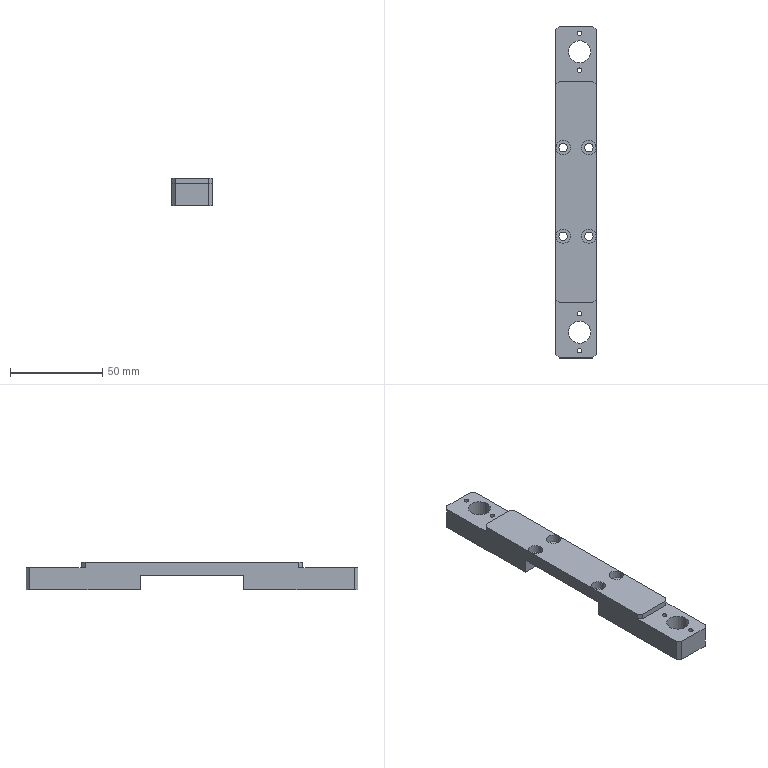Part | NX | 1 solid | 40 faces | box 22 x 180 x 15 mm | volume 41490 mm3 | plane 26 | cylinder 14 | commonest cylinder face diameters 2.5 x4 4.5 x4 7.8 x4 12 x2
STEP:
#1=CARTESIAN_POINT('',(-9.,90.,4.5));
#2=VERTEX_POINT('',#1);
#3=CARTESIAN_POINT('',(-11.,88.,4.5));
#4=VERTEX_POINT('',#3);
#5=CARTESIAN_POINT('',(-11.,88.,4.5));
#6=DIRECTION('',(-0.7071,-0.7071,0.));
#7=VECTOR('',#6,1000.);
#8=LINE('',#5,#7);
#9=EDGE_CURVE('',#2,#4,#8,.T.);
#10=ORIENTED_EDGE('',*,*,#9,.F.);
#11=CARTESIAN_POINT('',(-9.,90.,-7.5));
#12=VERTEX_POINT('',#11);
#13=CARTESIAN_POINT('',(-9.,90.,7.5));
#14=DIRECTION('',(0.,0.,1.));
#15=VECTOR('',#14,1000.);
#16=LINE('',#13,#15);
#17=EDGE_CURVE('',#12,#2,#16,.T.);
#18=ORIENTED_EDGE('',*,*,#17,.F.);
#19=CARTESIAN_POINT('',(-11.,88.,-7.5));
#20=VERTEX_POINT('',#19);
#21=CARTESIAN_POINT('',(-11.,88.,-7.5));
#22=DIRECTION('',(0.7071,0.7071,0.));
#23=VECTOR('',#22,1000.);
#24=LINE('',#21,#23);
#25=EDGE_CURVE('',#20,#12,#24,.T.);
#26=ORIENTED_EDGE('',*,*,#25,.F.);
#27=CARTESIAN_POINT('',(-11.,88.,7.5));
#28=DIRECTION('',(0.,0.,-1.));
#29=VECTOR('',#28,1000.);
#30=LINE('',#27,#29);
#31=EDGE_CURVE('',#4,#20,#30,.T.);
#32=ORIENTED_EDGE('',*,*,#31,.F.);
#33=EDGE_LOOP('',(#10,#18,#26,#32));
#34=FACE_BOUND('',#33,.T.);
#35=CARTESIAN_POINT('',(-11.,88.,7.5));
#36=DIRECTION('',(0.7071,-0.7071,0.));
#37=DIRECTION('',(0.,0.,-1.));
#38=AXIS2_PLACEMENT_3D('',#35,#36,#37);
#39=PLANE('',#38);
#40=ADVANCED_FACE('',(#34),#39,.F.);
#41=CARTESIAN_POINT('',(11.,88.,4.5));
#42=VERTEX_POINT('',#41);
#43=CARTESIAN_POINT('',(9.,90.,4.5));
#44=VERTEX_POINT('',#43);
#45=CARTESIAN_POINT('',(9.,90.,4.5));
#46=DIRECTION('',(-0.7071,0.7071,0.));
#47=VECTOR('',#46,1000.);
#48=LINE('',#45,#47);
#49=EDGE_CURVE('',#42,#44,#48,.T.);
#50=ORIENTED_EDGE('',*,*,#49,.F.);
#51=CARTESIAN_POINT('',(11.,88.,-7.5));
#52=VERTEX_POINT('',#51);
#53=CARTESIAN_POINT('',(11.,88.,7.5));
#54=DIRECTION('',(0.,0.,1.));
#55=VECTOR('',#54,1000.);
#56=LINE('',#53,#55);
#57=EDGE_CURVE('',#52,#42,#56,.T.);
#58=ORIENTED_EDGE('',*,*,#57,.F.);
#59=CARTESIAN_POINT('',(9.,90.,-7.5));
#60=VERTEX_POINT('',#59);
#61=CARTESIAN_POINT('',(9.,90.,-7.5));
#62=DIRECTION('',(0.7071,-0.7071,0.));
#63=VECTOR('',#62,1000.);
#64=LINE('',#61,#63);
#65=EDGE_CURVE('',#60,#52,#64,.T.);
#66=ORIENTED_EDGE('',*,*,#65,.F.);
#67=CARTESIAN_POINT('',(9.,90.,7.5));
#68=DIRECTION('',(0.,0.,-1.));
#69=VECTOR('',#68,1000.);
#70=LINE('',#67,#69);
#71=EDGE_CURVE('',#44,#60,#70,.T.);
#72=ORIENTED_EDGE('',*,*,#71,.F.);
#73=EDGE_LOOP('',(#50,#58,#66,#72));
#74=FACE_BOUND('',#73,.T.);
#75=CARTESIAN_POINT('',(9.,90.,7.5));
#76=DIRECTION('',(-0.7071,-0.7071,0.));
#77=DIRECTION('',(0.,0.,-1.));
#78=AXIS2_PLACEMENT_3D('',#75,#76,#77);
#79=PLANE('',#78);
#80=ADVANCED_FACE('',(#74),#79,.F.);
#81=CARTESIAN_POINT('',(-11.,-88.,4.5));
#82=VERTEX_POINT('',#81);
#83=CARTESIAN_POINT('',(-9.,-90.,4.5));
#84=VERTEX_POINT('',#83);
#85=CARTESIAN_POINT('',(-9.,-90.,4.5));
#86=DIRECTION('',(0.7071,-0.7071,0.));
#87=VECTOR('',#86,1000.);
#88=LINE('',#85,#87);
#89=EDGE_CURVE('',#82,#84,#88,.T.);
#90=ORIENTED_EDGE('',*,*,#89,.F.);
#91=CARTESIAN_POINT('',(-11.,-88.,-7.5));
#92=VERTEX_POINT('',#91);
#93=CARTESIAN_POINT('',(-11.,-88.,7.5));
#94=DIRECTION('',(0.,0.,1.));
#95=VECTOR('',#94,1000.);
#96=LINE('',#93,#95);
#97=EDGE_CURVE('',#92,#82,#96,.T.);
#98=ORIENTED_EDGE('',*,*,#97,.F.);
#99=CARTESIAN_POINT('',(-9.,-90.,-7.5));
#100=VERTEX_POINT('',#99);
#101=CARTESIAN_POINT('',(-9.,-90.,-7.5));
#102=DIRECTION('',(-0.7071,0.7071,0.));
#103=VECTOR('',#102,1000.);
#104=LINE('',#101,#103);
#105=EDGE_CURVE('',#100,#92,#104,.T.);
#106=ORIENTED_EDGE('',*,*,#105,.F.);
#107=CARTESIAN_POINT('',(-9.,-90.,7.5));
#108=DIRECTION('',(0.,0.,-1.));
#109=VECTOR('',#108,1000.);
#110=LINE('',#107,#109);
#111=EDGE_CURVE('',#84,#100,#110,.T.);
#112=ORIENTED_EDGE('',*,*,#111,.F.);
#113=EDGE_LOOP('',(#90,#98,#106,#112));
#114=FACE_BOUND('',#113,.T.);
#115=CARTESIAN_POINT('',(-9.,-90.,7.5));
#116=DIRECTION('',(0.7071,0.7071,0.));
#117=DIRECTION('',(0.,0.,-1.));
#118=AXIS2_PLACEMENT_3D('',#115,#116,#117);
#119=PLANE('',#118);
#120=ADVANCED_FACE('',(#114),#119,.F.);
#121=CARTESIAN_POINT('',(9.,-90.,4.5));
#122=VERTEX_POINT('',#121);
#123=CARTESIAN_POINT('',(11.,-88.,4.5));
#124=VERTEX_POINT('',#123);
#125=CARTESIAN_POINT('',(11.,-88.,4.5));
#126=DIRECTION('',(0.7071,0.7071,0.));
#127=VECTOR('',#126,1000.);
#128=LINE('',#125,#127);
#129=EDGE_CURVE('',#122,#124,#128,.T.);
#130=ORIENTED_EDGE('',*,*,#129,.F.);
#131=CARTESIAN_POINT('',(9.,-90.,-7.5));
#132=VERTEX_POINT('',#131);
#133=CARTESIAN_POINT('',(9.,-90.,7.5));
#134=DIRECTION('',(0.,0.,1.));
#135=VECTOR('',#134,1000.);
#136=LINE('',#133,#135);
#137=EDGE_CURVE('',#132,#122,#136,.T.);
#138=ORIENTED_EDGE('',*,*,#137,.F.);
#139=CARTESIAN_POINT('',(11.,-88.,-7.5));
#140=VERTEX_POINT('',#139);
#141=CARTESIAN_POINT('',(11.,-88.,-7.5));
#142=DIRECTION('',(-0.7071,-0.7071,0.));
#143=VECTOR('',#142,1000.);
#144=LINE('',#141,#143);
#145=EDGE_CURVE('',#140,#132,#144,.T.);
#146=ORIENTED_EDGE('',*,*,#145,.F.);
#147=CARTESIAN_POINT('',(11.,-88.,7.5));
#148=DIRECTION('',(0.,0.,-1.));
#149=VECTOR('',#148,1000.);
#150=LINE('',#147,#149);
#151=EDGE_CURVE('',#124,#140,#150,.T.);
#152=ORIENTED_EDGE('',*,*,#151,.F.);
#153=EDGE_LOOP('',(#130,#138,#146,#152));
#154=FACE_BOUND('',#153,.T.);
#155=CARTESIAN_POINT('',(11.,-88.,7.5));
#156=DIRECTION('',(-0.7071,0.7071,0.));
#157=DIRECTION('',(0.,0.,-1.));
#158=AXIS2_PLACEMENT_3D('',#155,#156,#157);
#159=PLANE('',#158);
#160=ADVANCED_FACE('',(#154),#159,.F.);
#161=CARTESIAN_POINT('',(-9.,-60.,4.5));
#162=VERTEX_POINT('',#161);
#163=CARTESIAN_POINT('',(-11.,-58.,4.5));
#164=VERTEX_POINT('',#163);
#165=CARTESIAN_POINT('',(-34.5,-34.5,4.5));
#166=DIRECTION('',(-0.7071,0.7071,0.));
#167=VECTOR('',#166,1000.);
#168=LINE('',#165,#167);
#169=EDGE_CURVE('',#162,#164,#168,.T.);
#170=ORIENTED_EDGE('',*,*,#169,.F.);
#171=CARTESIAN_POINT('',(-9.,-60.,7.5));
#172=VERTEX_POINT('',#171);
#173=CARTESIAN_POINT('',(-9.,-60.,4.5));
#174=DIRECTION('',(0.,0.,-1.));
#175=VECTOR('',#174,1000.);
#176=LINE('',#173,#175);
#177=EDGE_CURVE('',#172,#162,#176,.T.);
#178=ORIENTED_EDGE('',*,*,#177,.F.);
#179=CARTESIAN_POINT('',(-11.,-58.,7.5));
#180=VERTEX_POINT('',#179);
#181=CARTESIAN_POINT('',(-34.5,-34.5,7.5));
#182=DIRECTION('',(0.7071,-0.7071,0.));
#183=VECTOR('',#182,1000.);
#184=LINE('',#181,#183);
#185=EDGE_CURVE('',#180,#172,#184,.T.);
#186=ORIENTED_EDGE('',*,*,#185,.F.);
#187=CARTESIAN_POINT('',(-11.,-58.,7.5));
#188=DIRECTION('',(0.,0.,1.));
#189=VECTOR('',#188,1000.);
#190=LINE('',#187,#189);
#191=EDGE_CURVE('',#164,#180,#190,.T.);
#192=ORIENTED_EDGE('',*,*,#191,.F.);
#193=EDGE_LOOP('',(#170,#178,#186,#192));
#194=FACE_BOUND('',#193,.T.);
#195=CARTESIAN_POINT('',(-11.,-58.,7.5));
#196=DIRECTION('',(0.7071,0.7071,0.));
#197=DIRECTION('',(0.,0.,1.));
#198=AXIS2_PLACEMENT_3D('',#195,#196,#197);
#199=PLANE('',#198);
#200=ADVANCED_FACE('',(#194),#199,.F.);
#201=CARTESIAN_POINT('',(11.,-58.,4.5));
#202=VERTEX_POINT('',#201);
#203=CARTESIAN_POINT('',(9.,-60.,4.5));
#204=VERTEX_POINT('',#203);
#205=CARTESIAN_POINT('',(34.5,-34.5,4.5));
#206=DIRECTION('',(-0.7071,-0.7071,0.));
#207=VECTOR('',#206,1000.);
#208=LINE('',#205,#207);
#209=EDGE_CURVE('',#202,#204,#208,.T.);
#210=ORIENTED_EDGE('',*,*,#209,.F.);
#211=CARTESIAN_POINT('',(11.,-58.,7.5));
#212=VERTEX_POINT('',#211);
#213=CARTESIAN_POINT('',(11.,-58.,7.5));
#214=DIRECTION('',(0.,0.,-1.));
#215=VECTOR('',#214,1000.);
#216=LINE('',#213,#215);
#217=EDGE_CURVE('',#212,#202,#216,.T.);
#218=ORIENTED_EDGE('',*,*,#217,.F.);
#219=CARTESIAN_POINT('',(9.,-60.,7.5));
#220=VERTEX_POINT('',#219);
#221=CARTESIAN_POINT('',(34.5,-34.5,7.5));
#222=DIRECTION('',(0.7071,0.7071,0.));
#223=VECTOR('',#222,1000.);
#224=LINE('',#221,#223);
#225=EDGE_CURVE('',#220,#212,#224,.T.);
#226=ORIENTED_EDGE('',*,*,#225,.F.);
#227=CARTESIAN_POINT('',(9.,-60.,4.5));
#228=DIRECTION('',(0.,0.,1.));
#229=VECTOR('',#228,1000.);
#230=LINE('',#227,#229);
#231=EDGE_CURVE('',#204,#220,#230,.T.);
#232=ORIENTED_EDGE('',*,*,#231,.F.);
#233=EDGE_LOOP('',(#210,#218,#226,#232));
#234=FACE_BOUND('',#233,.T.);
#235=CARTESIAN_POINT('',(9.,-60.,4.5));
#236=DIRECTION('',(-0.7071,0.7071,0.));
#237=DIRECTION('',(0.,0.,1.));
#238=AXIS2_PLACEMENT_3D('',#235,#236,#237);
#239=PLANE('',#238);
#240=ADVANCED_FACE('',(#234),#239,.F.);
#241=CARTESIAN_POINT('',(-11.,58.,4.5));
#242=VERTEX_POINT('',#241);
#243=CARTESIAN_POINT('',(-9.,60.,4.5));
#244=VERTEX_POINT('',#243);
#245=CARTESIAN_POINT('',(-34.5,34.5,4.5));
#246=DIRECTION('',(0.7071,0.7071,0.));
#247=VECTOR('',#246,1000.);
#248=LINE('',#245,#247);
#249=EDGE_CURVE('',#242,#244,#248,.T.);
#250=ORIENTED_EDGE('',*,*,#249,.F.);
#251=CARTESIAN_POINT('',(-11.,58.,7.5));
#252=VERTEX_POINT('',#251);
#253=CARTESIAN_POINT('',(-11.,58.,7.5));
#254=DIRECTION('',(0.,0.,-1.));
#255=VECTOR('',#254,1000.);
#256=LINE('',#253,#255);
#257=EDGE_CURVE('',#252,#242,#256,.T.);
#258=ORIENTED_EDGE('',*,*,#257,.F.);
#259=CARTESIAN_POINT('',(-9.,60.,7.5));
#260=VERTEX_POINT('',#259);
#261=CARTESIAN_POINT('',(-34.5,34.5,7.5));
#262=DIRECTION('',(-0.7071,-0.7071,0.));
#263=VECTOR('',#262,1000.);
#264=LINE('',#261,#263);
#265=EDGE_CURVE('',#260,#252,#264,.T.);
#266=ORIENTED_EDGE('',*,*,#265,.F.);
#267=CARTESIAN_POINT('',(-9.,60.,4.5));
#268=DIRECTION('',(0.,0.,1.));
#269=VECTOR('',#268,1000.);
#270=LINE('',#267,#269);
#271=EDGE_CURVE('',#244,#260,#270,.T.);
#272=ORIENTED_EDGE('',*,*,#271,.F.);
#273=EDGE_LOOP('',(#250,#258,#266,#272));
#274=FACE_BOUND('',#273,.T.);
#275=CARTESIAN_POINT('',(-9.,60.,4.5));
#276=DIRECTION('',(0.7071,-0.7071,0.));
#277=DIRECTION('',(0.,0.,1.));
#278=AXIS2_PLACEMENT_3D('',#275,#276,#277);
#279=PLANE('',#278);
#280=ADVANCED_FACE('',(#274),#279,.F.);
#281=CARTESIAN_POINT('',(9.,60.,4.5));
#282=VERTEX_POINT('',#281);
#283=CARTESIAN_POINT('',(11.,58.,4.5));
#284=VERTEX_POINT('',#283);
#285=CARTESIAN_POINT('',(34.5,34.5,4.5));
#286=DIRECTION('',(0.7071,-0.7071,0.));
#287=VECTOR('',#286,1000.);
#288=LINE('',#285,#287);
#289=EDGE_CURVE('',#282,#284,#288,.T.);
#290=ORIENTED_EDGE('',*,*,#289,.F.);
#291=CARTESIAN_POINT('',(9.,60.,7.5));
#292=VERTEX_POINT('',#291);
#293=CARTESIAN_POINT('',(9.,60.,4.5));
#294=DIRECTION('',(0.,0.,-1.));
#295=VECTOR('',#294,1000.);
#296=LINE('',#293,#295);
#297=EDGE_CURVE('',#292,#282,#296,.T.);
#298=ORIENTED_EDGE('',*,*,#297,.F.);
#299=CARTESIAN_POINT('',(11.,58.,7.5));
#300=VERTEX_POINT('',#299);
#301=CARTESIAN_POINT('',(34.5,34.5,7.5));
#302=DIRECTION('',(-0.7071,0.7071,0.));
#303=VECTOR('',#302,1000.);
#304=LINE('',#301,#303);
#305=EDGE_CURVE('',#300,#292,#304,.T.);
#306=ORIENTED_EDGE('',*,*,#305,.F.);
#307=CARTESIAN_POINT('',(11.,58.,7.5));
#308=DIRECTION('',(0.,0.,1.));
#309=VECTOR('',#308,1000.);
#310=LINE('',#307,#309);
#311=EDGE_CURVE('',#284,#300,#310,.T.);
#312=ORIENTED_EDGE('',*,*,#311,.F.);
#313=EDGE_LOOP('',(#290,#298,#306,#312));
#314=FACE_BOUND('',#313,.T.);
#315=CARTESIAN_POINT('',(11.,58.,7.5));
#316=DIRECTION('',(-0.7071,-0.7071,0.));
#317=DIRECTION('',(0.,0.,1.));
#318=AXIS2_PLACEMENT_3D('',#315,#316,#317);
#319=PLANE('',#318);
#320=ADVANCED_FACE('',(#314),#319,.F.);
#321=CARTESIAN_POINT('',(-11.,28.05,-7.5));
#322=VERTEX_POINT('',#321);
#323=CARTESIAN_POINT('',(11.,28.05,-7.5));
#324=VERTEX_POINT('',#323);
#325=CARTESIAN_POINT('',(11.,28.05,-7.5));
#326=DIRECTION('',(1.,0.,0.));
#327=VECTOR('',#326,1000.);
#328=LINE('',#325,#327);
#329=EDGE_CURVE('',#322,#324,#328,.T.);
#330=ORIENTED_EDGE('',*,*,#329,.T.);
#331=CARTESIAN_POINT('',(11.,28.05,0.5));
#332=VERTEX_POINT('',#331);
#333=CARTESIAN_POINT('',(11.,28.05,0.5));
#334=DIRECTION('',(0.,0.,-1.));
#335=VECTOR('',#334,1000.);
#336=LINE('',#333,#335);
#337=EDGE_CURVE('',#332,#324,#336,.T.);
#338=ORIENTED_EDGE('',*,*,#337,.F.);
#339=CARTESIAN_POINT('',(-11.,28.05,0.5));
#340=VERTEX_POINT('',#339);
#341=CARTESIAN_POINT('',(11.,28.05,0.5));
#342=DIRECTION('',(1.,0.,0.));
#343=VECTOR('',#342,1000.);
#344=LINE('',#341,#343);
#345=EDGE_CURVE('',#340,#332,#344,.T.);
#346=ORIENTED_EDGE('',*,*,#345,.F.);
#347=CARTESIAN_POINT('',(-11.,28.05,0.5));
#348=DIRECTION('',(0.,0.,-1.));
#349=VECTOR('',#348,1000.);
#350=LINE('',#347,#349);
#351=EDGE_CURVE('',#340,#322,#350,.T.);
#352=ORIENTED_EDGE('',*,*,#351,.T.);
#353=EDGE_LOOP('',(#330,#338,#346,#352));
#354=FACE_BOUND('',#353,.T.);
#355=CARTESIAN_POINT('',(11.,28.05,0.5));
#356=DIRECTION('',(0.,1.,0.));
#357=DIRECTION('',(0.,0.,1.));
#358=AXIS2_PLACEMENT_3D('',#355,#356,#357);
#359=PLANE('',#358);
#360=ADVANCED_FACE('',(#354),#359,.F.);
#361=CARTESIAN_POINT('',(11.,-28.05,-7.5));
#362=VERTEX_POINT('',#361);
#363=CARTESIAN_POINT('',(-11.,-28.05,-7.5));
#364=VERTEX_POINT('',#363);
#365=CARTESIAN_POINT('',(11.,-28.05,-7.5));
#366=DIRECTION('',(-1.,0.,0.));
#367=VECTOR('',#366,1000.);
#368=LINE('',#365,#367);
#369=EDGE_CURVE('',#362,#364,#368,.T.);
#370=ORIENTED_EDGE('',*,*,#369,.T.);
#371=CARTESIAN_POINT('',(-11.,-28.05,0.5));
#372=VERTEX_POINT('',#371);
#373=CARTESIAN_POINT('',(-11.,-28.05,0.5));
#374=DIRECTION('',(0.,0.,-1.));
#375=VECTOR('',#374,1000.);
#376=LINE('',#373,#375);
#377=EDGE_CURVE('',#372,#364,#376,.T.);
#378=ORIENTED_EDGE('',*,*,#377,.F.);
#379=CARTESIAN_POINT('',(11.,-28.05,0.5));
#380=VERTEX_POINT('',#379);
#381=CARTESIAN_POINT('',(11.,-28.05,0.5));
#382=DIRECTION('',(-1.,0.,0.));
#383=VECTOR('',#382,1000.);
#384=LINE('',#381,#383);
#385=EDGE_CURVE('',#380,#372,#384,.T.);
#386=ORIENTED_EDGE('',*,*,#385,.F.);
#387=CARTESIAN_POINT('',(11.,-28.05,0.5));
#388=DIRECTION('',(0.,0.,-1.));
#389=VECTOR('',#388,1000.);
#390=LINE('',#387,#389);
#391=EDGE_CURVE('',#380,#362,#390,.T.);
#392=ORIENTED_EDGE('',*,*,#391,.T.);
#393=EDGE_LOOP('',(#370,#378,#386,#392));
#394=FACE_BOUND('',#393,.T.);
#395=CARTESIAN_POINT('',(11.,-28.05,0.5));
#396=DIRECTION('',(0.,-1.,0.));
#397=DIRECTION('',(0.,0.,-1.));
#398=AXIS2_PLACEMENT_3D('',#395,#396,#397);
#399=PLANE('',#398);
#400=ADVANCED_FACE('',(#394),#399,.F.);
#401=CARTESIAN_POINT('',(-4.75,-24.,0.5));
#402=VERTEX_POINT('',#401);
#403=CARTESIAN_POINT('',(-7.,-24.,0.5));
#404=DIRECTION('',(0.,0.,-1.));
#405=DIRECTION('',(1.,0.,0.));
#406=AXIS2_PLACEMENT_3D('',#403,#404,#405);
#407=CIRCLE('',#406,2.25);
#408=EDGE_CURVE('',#402,#402,#407,.T.);
#409=ORIENTED_EDGE('',*,*,#408,.F.);
#410=EDGE_LOOP('',(#409));
#411=FACE_BOUND('',#410,.T.);
#412=CARTESIAN_POINT('',(9.25,24.,0.5));
#413=VERTEX_POINT('',#412);
#414=CARTESIAN_POINT('',(7.,24.,0.5));
#415=DIRECTION('',(0.,0.,-1.));
#416=DIRECTION('',(1.,0.,0.));
#417=AXIS2_PLACEMENT_3D('',#414,#415,#416);
#418=CIRCLE('',#417,2.25);
#419=EDGE_CURVE('',#413,#413,#418,.T.);
#420=ORIENTED_EDGE('',*,*,#419,.F.);
#421=EDGE_LOOP('',(#420));
#422=FACE_BOUND('',#421,.T.);
#423=CARTESIAN_POINT('',(-11.,-28.05,0.5));
#424=DIRECTION('',(0.,1.,0.));
#425=VECTOR('',#424,1000.);
#426=LINE('',#423,#425);
#427=EDGE_CURVE('',#372,#340,#426,.T.);
#428=ORIENTED_EDGE('',*,*,#427,.T.);
#429=ORIENTED_EDGE('',*,*,#345,.T.);
#430=CARTESIAN_POINT('',(11.,-28.05,0.5));
#431=DIRECTION('',(0.,-1.,0.));
#432=VECTOR('',#431,1000.);
#433=LINE('',#430,#432);
#434=EDGE_CURVE('',#332,#380,#433,.T.);
#435=ORIENTED_EDGE('',*,*,#434,.T.);
#436=ORIENTED_EDGE('',*,*,#385,.T.);
#437=EDGE_LOOP('',(#428,#429,#435,#436));
#438=FACE_BOUND('',#437,.T.);
#439=CARTESIAN_POINT('',(-4.75,24.,0.5));
#440=VERTEX_POINT('',#439);
#441=CARTESIAN_POINT('',(-7.,24.,0.5));
#442=DIRECTION('',(0.,0.,-1.));
#443=DIRECTION('',(1.,0.,0.));
#444=AXIS2_PLACEMENT_3D('',#441,#442,#443);
#445=CIRCLE('',#444,2.25);
#446=EDGE_CURVE('',#440,#440,#445,.T.);
#447=ORIENTED_EDGE('',*,*,#446,.F.);
#448=EDGE_LOOP('',(#447));
#449=FACE_BOUND('',#448,.T.);
#450=CARTESIAN_POINT('',(9.25,-24.,0.5));
#451=VERTEX_POINT('',#450);
#452=CARTESIAN_POINT('',(7.,-24.,0.5));
#453=DIRECTION('',(0.,0.,-1.));
#454=DIRECTION('',(1.,0.,0.));
#455=AXIS2_PLACEMENT_3D('',#452,#453,#454);
#456=CIRCLE('',#455,2.25);
#457=EDGE_CURVE('',#451,#451,#456,.T.);
#458=ORIENTED_EDGE('',*,*,#457,.F.);
#459=EDGE_LOOP('',(#458));
#460=FACE_BOUND('',#459,.T.);
#461=CARTESIAN_POINT('',(0.,0.,0.5));
#462=DIRECTION('',(0.,0.,1.));
#463=DIRECTION('',(1.,0.,0.));
#464=AXIS2_PLACEMENT_3D('',#461,#462,#463);
#465=PLANE('',#464);
#466=ADVANCED_FACE('',(#411,#422,#438,#449,#460),#465,.F.);
#467=CARTESIAN_POINT('',(-11.,60.,7.5));
#468=DIRECTION('',(1.,0.,0.));
#469=VECTOR('',#468,1000.);
#470=LINE('',#467,#469);
#471=EDGE_CURVE('',#260,#292,#470,.T.);
#472=ORIENTED_EDGE('',*,*,#471,.T.);
#473=ORIENTED_EDGE('',*,*,#297,.T.);
#474=CARTESIAN_POINT('',(-11.,60.,4.5));
#475=DIRECTION('',(1.,0.,0.));
#476=VECTOR('',#475,1000.);
#477=LINE('',#474,#476);
#478=EDGE_CURVE('',#244,#282,#477,.T.);
#479=ORIENTED_EDGE('',*,*,#478,.F.);
#480=ORIENTED_EDGE('',*,*,#271,.T.);
#481=EDGE_LOOP('',(#472,#473,#479,#480));
#482=FACE_BOUND('',#481,.T.);
#483=CARTESIAN_POINT('',(-11.,60.,4.5));
#484=DIRECTION('',(0.,-1.,0.));
#485=DIRECTION('',(0.,0.,-1.));
#486=AXIS2_PLACEMENT_3D('',#483,#484,#485);
#487=PLANE('',#486);
#488=ADVANCED_FACE('',(#482),#487,.F.);
#489=CARTESIAN_POINT('',(-4.,76.,4.5));
#490=VERTEX_POINT('',#489);
#491=CARTESIAN_POINT('',(2.,76.,4.5));
#492=DIRECTION('',(0.,0.,1.));
#493=DIRECTION('',(-1.,0.,0.));
#494=AXIS2_PLACEMENT_3D('',#491,#492,#493);
#495=CIRCLE('',#494,6.);
#496=EDGE_CURVE('',#490,#490,#495,.T.);
#497=ORIENTED_EDGE('',*,*,#496,.F.);
#498=EDGE_LOOP('',(#497));
#499=FACE_BOUND('',#498,.T.);
#500=CARTESIAN_POINT('',(11.,90.,4.5));
#501=DIRECTION('',(0.,1.,0.));
#502=VECTOR('',#501,1000.);
#503=LINE('',#500,#502);
#504=EDGE_CURVE('',#284,#42,#503,.T.);
#505=ORIENTED_EDGE('',*,*,#504,.T.);
#506=ORIENTED_EDGE('',*,*,#49,.T.);
#507=CARTESIAN_POINT('',(-11.,90.,4.5));
#508=DIRECTION('',(-1.,0.,0.));
#509=VECTOR('',#508,1000.);
#510=LINE('',#507,#509);
#511=EDGE_CURVE('',#44,#2,#510,.T.);
#512=ORIENTED_EDGE('',*,*,#511,.T.);
#513=ORIENTED_EDGE('',*,*,#9,.T.);
#514=CARTESIAN_POINT('',(-11.,90.,4.5));
#515=DIRECTION('',(0.,-1.,0.));
#516=VECTOR('',#515,1000.);
#517=LINE('',#514,#516);
#518=EDGE_CURVE('',#4,#242,#517,.T.);
#519=ORIENTED_EDGE('',*,*,#518,.T.);
#520=ORIENTED_EDGE('',*,*,#249,.T.);
#521=ORIENTED_EDGE('',*,*,#478,.T.);
#522=ORIENTED_EDGE('',*,*,#289,.T.);
#523=EDGE_LOOP('',(#505,#506,#512,#513,#519,#520,#521,#522));
#524=FACE_BOUND('',#523,.T.);
#525=CARTESIAN_POINT('',(0.75,66.,4.5));
#526=VERTEX_POINT('',#525);
#527=CARTESIAN_POINT('',(2.,66.,4.5));
#528=DIRECTION('',(0.,0.,-1.));
#529=DIRECTION('',(-1.,0.,0.));
#530=AXIS2_PLACEMENT_3D('',#527,#528,#529);
#531=CIRCLE('',#530,1.25);
#532=EDGE_CURVE('',#526,#526,#531,.T.);
#533=ORIENTED_EDGE('',*,*,#532,.T.);
#534=EDGE_LOOP('',(#533));
#535=FACE_BOUND('',#534,.T.);
#536=CARTESIAN_POINT('',(0.75,86.,4.5));
#537=VERTEX_POINT('',#536);
#538=CARTESIAN_POINT('',(2.,86.,4.5));
#539=DIRECTION('',(0.,0.,-1.));
#540=DIRECTION('',(-1.,0.,0.));
#541=AXIS2_PLACEMENT_3D('',#538,#539,#540);
#542=CIRCLE('',#541,1.25);
#543=EDGE_CURVE('',#537,#537,#542,.T.);
#544=ORIENTED_EDGE('',*,*,#543,.T.);
#545=EDGE_LOOP('',(#544));
#546=FACE_BOUND('',#545,.T.);
#547=CARTESIAN_POINT('',(0.,0.,4.5));
#548=DIRECTION('',(0.,0.,-1.));
#549=DIRECTION('',(-1.,0.,0.));
#550=AXIS2_PLACEMENT_3D('',#547,#548,#549);
#551=PLANE('',#550);
#552=ADVANCED_FACE('',(#499,#524,#535,#546),#551,.F.);
#553=CARTESIAN_POINT('',(-11.,-60.,4.5));
#554=DIRECTION('',(-1.,0.,0.));
#555=VECTOR('',#554,1000.);
#556=LINE('',#553,#555);
#557=EDGE_CURVE('',#204,#162,#556,.T.);
#558=ORIENTED_EDGE('',*,*,#557,.F.);
#559=ORIENTED_EDGE('',*,*,#231,.T.);
#560=CARTESIAN_POINT('',(-11.,-60.,7.5));
#561=DIRECTION('',(-1.,0.,0.));
#562=VECTOR('',#561,1000.);
#563=LINE('',#560,#562);
#564=EDGE_CURVE('',#220,#172,#563,.T.);
#565=ORIENTED_EDGE('',*,*,#564,.T.);
#566=ORIENTED_EDGE('',*,*,#177,.T.);
#567=EDGE_LOOP('',(#558,#559,#565,#566));
#568=FACE_BOUND('',#567,.T.);
#569=CARTESIAN_POINT('',(-11.,-60.,4.5));
#570=DIRECTION('',(0.,1.,0.));
#571=DIRECTION('',(0.,0.,1.));
#572=AXIS2_PLACEMENT_3D('',#569,#570,#571);
#573=PLANE('',#572);
#574=ADVANCED_FACE('',(#568),#573,.F.);
#575=CARTESIAN_POINT('',(-4.,-76.,4.5));
#576=VERTEX_POINT('',#575);
#577=CARTESIAN_POINT('',(2.,-76.,4.5));
#578=DIRECTION('',(0.,0.,1.));
#579=DIRECTION('',(-1.,0.,0.));
#580=AXIS2_PLACEMENT_3D('',#577,#578,#579);
#581=CIRCLE('',#580,6.);
#582=EDGE_CURVE('',#576,#576,#581,.T.);
#583=ORIENTED_EDGE('',*,*,#582,.F.);
#584=EDGE_LOOP('',(#583));
#585=FACE_BOUND('',#584,.T.);
#586=CARTESIAN_POINT('',(-11.,-90.,4.5));
#587=DIRECTION('',(1.,0.,0.));
#588=VECTOR('',#587,1000.);
#589=LINE('',#586,#588);
#590=EDGE_CURVE('',#84,#122,#589,.T.);
#591=ORIENTED_EDGE('',*,*,#590,.T.);
#592=ORIENTED_EDGE('',*,*,#129,.T.);
#593=CARTESIAN_POINT('',(11.,-90.,4.5));
#594=DIRECTION('',(0.,1.,0.));
#595=VECTOR('',#594,1000.);
#596=LINE('',#593,#595);
#597=EDGE_CURVE('',#124,#202,#596,.T.);
#598=ORIENTED_EDGE('',*,*,#597,.T.);
#599=ORIENTED_EDGE('',*,*,#209,.T.);
#600=ORIENTED_EDGE('',*,*,#557,.T.);
#601=ORIENTED_EDGE('',*,*,#169,.T.);
#602=CARTESIAN_POINT('',(-11.,-90.,4.5));
#603=DIRECTION('',(0.,-1.,0.));
#604=VECTOR('',#603,1000.);
#605=LINE('',#602,#604);
#606=EDGE_CURVE('',#164,#82,#605,.T.);
#607=ORIENTED_EDGE('',*,*,#606,.T.);
#608=ORIENTED_EDGE('',*,*,#89,.T.);
#609=EDGE_LOOP('',(#591,#592,#598,#599,#600,#601,#607,#608));
#610=FACE_BOUND('',#609,.T.);
#611=CARTESIAN_POINT('',(0.75,-86.,4.5));
#612=VERTEX_POINT('',#611);
#613=CARTESIAN_POINT('',(2.,-86.,4.5));
#614=DIRECTION('',(0.,0.,-1.));
#615=DIRECTION('',(-1.,0.,0.));
#616=AXIS2_PLACEMENT_3D('',#613,#614,#615);
#617=CIRCLE('',#616,1.25);
#618=EDGE_CURVE('',#612,#612,#617,.T.);
#619=ORIENTED_EDGE('',*,*,#618,.T.);
#620=EDGE_LOOP('',(#619));
#621=FACE_BOUND('',#620,.T.);
#622=CARTESIAN_POINT('',(0.75,-66.,4.5));
#623=VERTEX_POINT('',#622);
#624=CARTESIAN_POINT('',(2.,-66.,4.5));
#625=DIRECTION('',(0.,0.,-1.));
#626=DIRECTION('',(-1.,0.,0.));
#627=AXIS2_PLACEMENT_3D('',#624,#625,#626);
#628=CIRCLE('',#627,1.25);
#629=EDGE_CURVE('',#623,#623,#628,.T.);
#630=ORIENTED_EDGE('',*,*,#629,.T.);
#631=EDGE_LOOP('',(#630));
#632=FACE_BOUND('',#631,.T.);
#633=CARTESIAN_POINT('',(0.,0.,4.5));
#634=DIRECTION('',(0.,0.,-1.));
#635=DIRECTION('',(-1.,0.,0.));
#636=AXIS2_PLACEMENT_3D('',#633,#634,#635);
#637=PLANE('',#636);
#638=ADVANCED_FACE('',(#585,#610,#621,#632),#637,.F.);
#639=CARTESIAN_POINT('',(-10.9,24.,3.1));
#640=VERTEX_POINT('',#639);
#641=CARTESIAN_POINT('',(-7.,24.,3.1));
#642=DIRECTION('',(0.,0.,1.));
#643=DIRECTION('',(-1.,0.,0.));
#644=AXIS2_PLACEMENT_3D('',#641,#642,#643);
#645=CIRCLE('',#644,3.9);
#646=EDGE_CURVE('',#640,#640,#645,.T.);
#647=ORIENTED_EDGE('',*,*,#646,.T.);
#648=EDGE_LOOP('',(#647));
#649=FACE_BOUND('',#648,.T.);
#650=CARTESIAN_POINT('',(-9.25,24.,3.1));
#651=VERTEX_POINT('',#650);
#652=CARTESIAN_POINT('',(-7.,24.,3.1));
#653=DIRECTION('',(0.,0.,1.));
#654=DIRECTION('',(-1.,0.,0.));
#655=AXIS2_PLACEMENT_3D('',#652,#653,#654);
#656=CIRCLE('',#655,2.25);
#657=EDGE_CURVE('',#651,#651,#656,.T.);
#658=ORIENTED_EDGE('',*,*,#657,.F.);
#659=EDGE_LOOP('',(#658));
#660=FACE_BOUND('',#659,.T.);
#661=CARTESIAN_POINT('',(-4.75,-24.,3.1));
#662=DIRECTION('',(0.,0.,-1.));
#663=DIRECTION('',(-1.,0.,0.));
#664=AXIS2_PLACEMENT_3D('',#661,#662,#663);
#665=PLANE('',#664);
#666=ADVANCED_FACE('',(#649,#660),#665,.F.);
#667=CARTESIAN_POINT('',(3.1,24.,3.1));
#668=VERTEX_POINT('',#667);
#669=CARTESIAN_POINT('',(7.,24.,3.1));
#670=DIRECTION('',(0.,0.,1.));
#671=DIRECTION('',(-1.,0.,0.));
#672=AXIS2_PLACEMENT_3D('',#669,#670,#671);
#673=CIRCLE('',#672,3.9);
#674=EDGE_CURVE('',#668,#668,#673,.T.);
#675=ORIENTED_EDGE('',*,*,#674,.T.);
#676=EDGE_LOOP('',(#675));
#677=FACE_BOUND('',#676,.T.);
#678=CARTESIAN_POINT('',(4.75,24.,3.1));
#679=VERTEX_POINT('',#678);
#680=CARTESIAN_POINT('',(7.,24.,3.1));
#681=DIRECTION('',(0.,0.,1.));
#682=DIRECTION('',(-1.,0.,0.));
#683=AXIS2_PLACEMENT_3D('',#680,#681,#682);
#684=CIRCLE('',#683,2.25);
#685=EDGE_CURVE('',#679,#679,#684,.T.);
#686=ORIENTED_EDGE('',*,*,#685,.F.);
#687=EDGE_LOOP('',(#686));
#688=FACE_BOUND('',#687,.T.);
#689=CARTESIAN_POINT('',(-4.75,-24.,3.1));
#690=DIRECTION('',(0.,0.,-1.));
#691=DIRECTION('',(-1.,0.,0.));
#692=AXIS2_PLACEMENT_3D('',#689,#690,#691);
#693=PLANE('',#692);
#694=ADVANCED_FACE('',(#677,#688),#693,.F.);
#695=CARTESIAN_POINT('',(3.1,-24.,3.1));
#696=VERTEX_POINT('',#695);
#697=CARTESIAN_POINT('',(7.,-24.,3.1));
#698=DIRECTION('',(0.,0.,1.));
#699=DIRECTION('',(-1.,0.,0.));
#700=AXIS2_PLACEMENT_3D('',#697,#698,#699);
#701=CIRCLE('',#700,3.9);
#702=EDGE_CURVE('',#696,#696,#701,.T.);
#703=ORIENTED_EDGE('',*,*,#702,.T.);
#704=EDGE_LOOP('',(#703));
#705=FACE_BOUND('',#704,.T.);
#706=CARTESIAN_POINT('',(4.75,-24.,3.1));
#707=VERTEX_POINT('',#706);
#708=CARTESIAN_POINT('',(7.,-24.,3.1));
#709=DIRECTION('',(0.,0.,1.));
#710=DIRECTION('',(-1.,0.,0.));
#711=AXIS2_PLACEMENT_3D('',#708,#709,#710);
#712=CIRCLE('',#711,2.25);
#713=EDGE_CURVE('',#707,#707,#712,.T.);
#714=ORIENTED_EDGE('',*,*,#713,.F.);
#715=EDGE_LOOP('',(#714));
#716=FACE_BOUND('',#715,.T.);
#717=CARTESIAN_POINT('',(-4.75,-24.,3.1));
#718=DIRECTION('',(0.,0.,-1.));
#719=DIRECTION('',(-1.,0.,0.));
#720=AXIS2_PLACEMENT_3D('',#717,#718,#719);
#721=PLANE('',#720);
#722=ADVANCED_FACE('',(#705,#716),#721,.F.);
#723=CARTESIAN_POINT('',(-3.1,-24.,3.1));
#724=VERTEX_POINT('',#723);
#725=CARTESIAN_POINT('',(-7.,-24.,3.1));
#726=DIRECTION('',(0.,0.,1.));
#727=DIRECTION('',(1.,0.,0.));
#728=AXIS2_PLACEMENT_3D('',#725,#726,#727);
#729=CIRCLE('',#728,3.9);
#730=EDGE_CURVE('',#724,#724,#729,.T.);
#731=ORIENTED_EDGE('',*,*,#730,.T.);
#732=EDGE_LOOP('',(#731));
#733=FACE_BOUND('',#732,.T.);
#734=CARTESIAN_POINT('',(-4.75,-24.,3.1));
#735=VERTEX_POINT('',#734);
#736=CARTESIAN_POINT('',(-7.,-24.,3.1));
#737=DIRECTION('',(0.,0.,1.));
#738=DIRECTION('',(1.,0.,0.));
#739=AXIS2_PLACEMENT_3D('',#736,#737,#738);
#740=CIRCLE('',#739,2.25);
#741=EDGE_CURVE('',#735,#735,#740,.T.);
#742=ORIENTED_EDGE('',*,*,#741,.F.);
#743=EDGE_LOOP('',(#742));
#744=FACE_BOUND('',#743,.T.);
#745=CARTESIAN_POINT('',(-4.75,-24.,3.1));
#746=DIRECTION('',(0.,0.,-1.));
#747=DIRECTION('',(-1.,0.,0.));
#748=AXIS2_PLACEMENT_3D('',#745,#746,#747);
#749=PLANE('',#748);
#750=ADVANCED_FACE('',(#733,#744),#749,.F.);
#751=CARTESIAN_POINT('',(-11.,90.,-7.5));
#752=DIRECTION('',(-1.,0.,0.));
#753=VECTOR('',#752,1000.);
#754=LINE('',#751,#753);
#755=EDGE_CURVE('',#60,#12,#754,.T.);
#756=ORIENTED_EDGE('',*,*,#755,.F.);
#757=ORIENTED_EDGE('',*,*,#65,.T.);
#758=CARTESIAN_POINT('',(11.,90.,-7.5));
#759=DIRECTION('',(0.,1.,0.));
#760=VECTOR('',#759,1000.);
#761=LINE('',#758,#760);
#762=EDGE_CURVE('',#324,#52,#761,.T.);
#763=ORIENTED_EDGE('',*,*,#762,.F.);
#764=ORIENTED_EDGE('',*,*,#329,.F.);
#765=CARTESIAN_POINT('',(-11.,90.,-7.5));
#766=DIRECTION('',(0.,-1.,0.));
#767=VECTOR('',#766,1000.);
#768=LINE('',#765,#767);
#769=EDGE_CURVE('',#20,#322,#768,.T.);
#770=ORIENTED_EDGE('',*,*,#769,.F.);
#771=ORIENTED_EDGE('',*,*,#25,.T.);
#772=EDGE_LOOP('',(#756,#757,#763,#764,#770,#771));
#773=FACE_BOUND('',#772,.T.);
#774=CARTESIAN_POINT('',(-4.,76.,-7.5));
#775=VERTEX_POINT('',#774);
#776=CARTESIAN_POINT('',(2.,76.,-7.5));
#777=DIRECTION('',(0.,0.,1.));
#778=DIRECTION('',(-1.,0.,0.));
#779=AXIS2_PLACEMENT_3D('',#776,#777,#778);
#780=CIRCLE('',#779,6.);
#781=EDGE_CURVE('',#775,#775,#780,.T.);
#782=ORIENTED_EDGE('',*,*,#781,.T.);
#783=EDGE_LOOP('',(#782));
#784=FACE_BOUND('',#783,.T.);
#785=CARTESIAN_POINT('',(0.75,66.,-7.5));
#786=VERTEX_POINT('',#785);
#787=CARTESIAN_POINT('',(2.,66.,-7.5));
#788=DIRECTION('',(0.,0.,-1.));
#789=DIRECTION('',(-1.,0.,0.));
#790=AXIS2_PLACEMENT_3D('',#787,#788,#789);
#791=CIRCLE('',#790,1.25);
#792=EDGE_CURVE('',#786,#786,#791,.T.);
#793=ORIENTED_EDGE('',*,*,#792,.F.);
#794=EDGE_LOOP('',(#793));
#795=FACE_BOUND('',#794,.T.);
#796=CARTESIAN_POINT('',(0.75,86.,-7.5));
#797=VERTEX_POINT('',#796);
#798=CARTESIAN_POINT('',(2.,86.,-7.5));
#799=DIRECTION('',(0.,0.,-1.));
#800=DIRECTION('',(-1.,0.,0.));
#801=AXIS2_PLACEMENT_3D('',#798,#799,#800);
#802=CIRCLE('',#801,1.25);
#803=EDGE_CURVE('',#797,#797,#802,.T.);
#804=ORIENTED_EDGE('',*,*,#803,.F.);
#805=EDGE_LOOP('',(#804));
#806=FACE_BOUND('',#805,.T.);
#807=CARTESIAN_POINT('',(0.,0.,-7.5));
#808=DIRECTION('',(0.,0.,1.));
#809=DIRECTION('',(1.,0.,0.));
#810=AXIS2_PLACEMENT_3D('',#807,#808,#809);
#811=PLANE('',#810);
#812=ADVANCED_FACE('',(#773,#784,#795,#806),#811,.F.);
#813=CARTESIAN_POINT('',(-3.1,-24.,7.5));
#814=VERTEX_POINT('',#813);
#815=CARTESIAN_POINT('',(-7.,-24.,7.5));
#816=DIRECTION('',(0.,0.,1.));
#817=DIRECTION('',(1.,0.,0.));
#818=AXIS2_PLACEMENT_3D('',#815,#816,#817);
#819=CIRCLE('',#818,3.9);
#820=EDGE_CURVE('',#814,#814,#819,.T.);
#821=ORIENTED_EDGE('',*,*,#820,.F.);
#822=EDGE_LOOP('',(#821));
#823=FACE_BOUND('',#822,.T.);
#824=CARTESIAN_POINT('',(10.9,-24.,7.5));
#825=VERTEX_POINT('',#824);
#826=CARTESIAN_POINT('',(7.,-24.,7.5));
#827=DIRECTION('',(0.,0.,1.));
#828=DIRECTION('',(1.,0.,0.));
#829=AXIS2_PLACEMENT_3D('',#826,#827,#828);
#830=CIRCLE('',#829,3.9);
#831=EDGE_CURVE('',#825,#825,#830,.T.);
#832=ORIENTED_EDGE('',*,*,#831,.F.);
#833=EDGE_LOOP('',(#832));
#834=FACE_BOUND('',#833,.T.);
#835=CARTESIAN_POINT('',(10.9,24.,7.5));
#836=VERTEX_POINT('',#835);
#837=CARTESIAN_POINT('',(7.,24.,7.5));
#838=DIRECTION('',(0.,0.,1.));
#839=DIRECTION('',(1.,0.,0.));
#840=AXIS2_PLACEMENT_3D('',#837,#838,#839);
#841=CIRCLE('',#840,3.9);
#842=EDGE_CURVE('',#836,#836,#841,.T.);
#843=ORIENTED_EDGE('',*,*,#842,.F.);
#844=EDGE_LOOP('',(#843));
#845=FACE_BOUND('',#844,.T.);
#846=CARTESIAN_POINT('',(-3.1,24.,7.5));
#847=VERTEX_POINT('',#846);
#848=CARTESIAN_POINT('',(-7.,24.,7.5));
#849=DIRECTION('',(0.,0.,1.));
#850=DIRECTION('',(1.,0.,0.));
#851=AXIS2_PLACEMENT_3D('',#848,#849,#850);
#852=CIRCLE('',#851,3.9);
#853=EDGE_CURVE('',#847,#847,#852,.T.);
#854=ORIENTED_EDGE('',*,*,#853,.F.);
#855=EDGE_LOOP('',(#854));
#856=FACE_BOUND('',#855,.T.);
#857=CARTESIAN_POINT('',(11.,90.,7.5));
#858=DIRECTION('',(0.,1.,0.));
#859=VECTOR('',#858,1000.);
#860=LINE('',#857,#859);
#861=EDGE_CURVE('',#212,#300,#860,.T.);
#862=ORIENTED_EDGE('',*,*,#861,.T.);
#863=ORIENTED_EDGE('',*,*,#305,.T.);
#864=ORIENTED_EDGE('',*,*,#471,.F.);
#865=ORIENTED_EDGE('',*,*,#265,.T.);
#866=CARTESIAN_POINT('',(-11.,90.,7.5));
#867=DIRECTION('',(0.,-1.,0.));
#868=VECTOR('',#867,1000.);
#869=LINE('',#866,#868);
#870=EDGE_CURVE('',#252,#180,#869,.T.);
#871=ORIENTED_EDGE('',*,*,#870,.T.);
#872=ORIENTED_EDGE('',*,*,#185,.T.);
#873=ORIENTED_EDGE('',*,*,#564,.F.);
#874=ORIENTED_EDGE('',*,*,#225,.T.);
#875=EDGE_LOOP('',(#862,#863,#864,#865,#871,#872,#873,#874));
#876=FACE_BOUND('',#875,.T.);
#877=CARTESIAN_POINT('',(0.,0.,7.5));
#878=DIRECTION('',(0.,0.,1.));
#879=DIRECTION('',(1.,0.,0.));
#880=AXIS2_PLACEMENT_3D('',#877,#878,#879);
#881=PLANE('',#880);
#882=ADVANCED_FACE('',(#823,#834,#845,#856,#876),#881,.T.);
#883=CARTESIAN_POINT('',(-11.,-90.,-7.5));
#884=DIRECTION('',(1.,0.,0.));
#885=VECTOR('',#884,1000.);
#886=LINE('',#883,#885);
#887=EDGE_CURVE('',#100,#132,#886,.T.);
#888=ORIENTED_EDGE('',*,*,#887,.T.);
#889=ORIENTED_EDGE('',*,*,#137,.T.);
#890=ORIENTED_EDGE('',*,*,#590,.F.);
#891=ORIENTED_EDGE('',*,*,#111,.T.);
#892=EDGE_LOOP('',(#888,#889,#890,#891));
#893=FACE_BOUND('',#892,.T.);
#894=CARTESIAN_POINT('',(-11.,-90.,7.5));
#895=DIRECTION('',(0.,1.,0.));
#896=DIRECTION('',(0.,0.,1.));
#897=AXIS2_PLACEMENT_3D('',#894,#895,#896);
#898=PLANE('',#897);
#899=ADVANCED_FACE('',(#893),#898,.F.);
#900=ORIENTED_EDGE('',*,*,#870,.F.);
#901=ORIENTED_EDGE('',*,*,#257,.T.);
#902=ORIENTED_EDGE('',*,*,#518,.F.);
#903=ORIENTED_EDGE('',*,*,#31,.T.);
#904=ORIENTED_EDGE('',*,*,#769,.T.);
#905=ORIENTED_EDGE('',*,*,#351,.F.);
#906=ORIENTED_EDGE('',*,*,#427,.F.);
#907=ORIENTED_EDGE('',*,*,#377,.T.);
#908=CARTESIAN_POINT('',(-11.,90.,-7.5));
#909=DIRECTION('',(0.,-1.,0.));
#910=VECTOR('',#909,1000.);
#911=LINE('',#908,#910);
#912=EDGE_CURVE('',#364,#92,#911,.T.);
#913=ORIENTED_EDGE('',*,*,#912,.T.);
#914=ORIENTED_EDGE('',*,*,#97,.T.);
#915=ORIENTED_EDGE('',*,*,#606,.F.);
#916=ORIENTED_EDGE('',*,*,#191,.T.);
#917=EDGE_LOOP('',(#900,#901,#902,#903,#904,#905,#906,#907,#913,#914,#915,#916));
#918=FACE_BOUND('',#917,.T.);
#919=CARTESIAN_POINT('',(-11.,90.,7.5));
#920=DIRECTION('',(1.,0.,0.));
#921=DIRECTION('',(0.,1.,0.));
#922=AXIS2_PLACEMENT_3D('',#919,#920,#921);
#923=PLANE('',#922);
#924=ADVANCED_FACE('',(#918),#923,.F.);
#925=ORIENTED_EDGE('',*,*,#511,.F.);
#926=ORIENTED_EDGE('',*,*,#71,.T.);
#927=ORIENTED_EDGE('',*,*,#755,.T.);
#928=ORIENTED_EDGE('',*,*,#17,.T.);
#929=EDGE_LOOP('',(#925,#926,#927,#928));
#930=FACE_BOUND('',#929,.T.);
#931=CARTESIAN_POINT('',(-11.,90.,7.5));
#932=DIRECTION('',(0.,-1.,0.));
#933=DIRECTION('',(0.,0.,-1.));
#934=AXIS2_PLACEMENT_3D('',#931,#932,#933);
#935=PLANE('',#934);
#936=ADVANCED_FACE('',(#930),#935,.F.);
#937=ORIENTED_EDGE('',*,*,#504,.F.);
#938=ORIENTED_EDGE('',*,*,#311,.T.);
#939=ORIENTED_EDGE('',*,*,#861,.F.);
#940=ORIENTED_EDGE('',*,*,#217,.T.);
#941=ORIENTED_EDGE('',*,*,#597,.F.);
#942=ORIENTED_EDGE('',*,*,#151,.T.);
#943=CARTESIAN_POINT('',(11.,90.,-7.5));
#944=DIRECTION('',(0.,1.,0.));
#945=VECTOR('',#944,1000.);
#946=LINE('',#943,#945);
#947=EDGE_CURVE('',#140,#362,#946,.T.);
#948=ORIENTED_EDGE('',*,*,#947,.T.);
#949=ORIENTED_EDGE('',*,*,#391,.F.);
#950=ORIENTED_EDGE('',*,*,#434,.F.);
#951=ORIENTED_EDGE('',*,*,#337,.T.);
#952=ORIENTED_EDGE('',*,*,#762,.T.);
#953=ORIENTED_EDGE('',*,*,#57,.T.);
#954=EDGE_LOOP('',(#937,#938,#939,#940,#941,#942,#948,#949,#950,#951,#952,#953));
#955=FACE_BOUND('',#954,.T.);
#956=CARTESIAN_POINT('',(11.,90.,7.5));
#957=DIRECTION('',(-1.,0.,0.));
#958=DIRECTION('',(0.,-1.,0.));
#959=AXIS2_PLACEMENT_3D('',#956,#957,#958);
#960=PLANE('',#959);
#961=ADVANCED_FACE('',(#955),#960,.F.);
#962=ORIENTED_EDGE('',*,*,#947,.F.);
#963=ORIENTED_EDGE('',*,*,#145,.T.);
#964=ORIENTED_EDGE('',*,*,#887,.F.);
#965=ORIENTED_EDGE('',*,*,#105,.T.);
#966=ORIENTED_EDGE('',*,*,#912,.F.);
#967=ORIENTED_EDGE('',*,*,#369,.F.);
#968=EDGE_LOOP('',(#962,#963,#964,#965,#966,#967));
#969=FACE_BOUND('',#968,.T.);
#970=CARTESIAN_POINT('',(0.75,-66.,-7.5));
#971=VERTEX_POINT('',#970);
#972=CARTESIAN_POINT('',(2.,-66.,-7.5));
#973=DIRECTION('',(0.,0.,-1.));
#974=DIRECTION('',(-1.,0.,0.));
#975=AXIS2_PLACEMENT_3D('',#972,#973,#974);
#976=CIRCLE('',#975,1.25);
#977=EDGE_CURVE('',#971,#971,#976,.T.);
#978=ORIENTED_EDGE('',*,*,#977,.F.);
#979=EDGE_LOOP('',(#978));
#980=FACE_BOUND('',#979,.T.);
#981=CARTESIAN_POINT('',(0.75,-86.,-7.5));
#982=VERTEX_POINT('',#981);
#983=CARTESIAN_POINT('',(2.,-86.,-7.5));
#984=DIRECTION('',(0.,0.,-1.));
#985=DIRECTION('',(-1.,0.,0.));
#986=AXIS2_PLACEMENT_3D('',#983,#984,#985);
#987=CIRCLE('',#986,1.25);
#988=EDGE_CURVE('',#982,#982,#987,.T.);
#989=ORIENTED_EDGE('',*,*,#988,.F.);
#990=EDGE_LOOP('',(#989));
#991=FACE_BOUND('',#990,.T.);
#992=CARTESIAN_POINT('',(8.,-76.,-7.5));
#993=VERTEX_POINT('',#992);
#994=CARTESIAN_POINT('',(2.,-76.,-7.5));
#995=DIRECTION('',(0.,0.,1.));
#996=DIRECTION('',(1.,0.,0.));
#997=AXIS2_PLACEMENT_3D('',#994,#995,#996);
#998=CIRCLE('',#997,6.);
#999=EDGE_CURVE('',#993,#993,#998,.T.);
#1000=ORIENTED_EDGE('',*,*,#999,.T.);
#1001=EDGE_LOOP('',(#1000));
#1002=FACE_BOUND('',#1001,.T.);
#1003=CARTESIAN_POINT('',(0.,0.,-7.5));
#1004=DIRECTION('',(0.,0.,1.));
#1005=DIRECTION('',(1.,0.,0.));
#1006=AXIS2_PLACEMENT_3D('',#1003,#1004,#1005);
#1007=PLANE('',#1006);
#1008=ADVANCED_FACE('',(#969,#980,#991,#1002),#1007,.F.);
#1009=ORIENTED_EDGE('',*,*,#408,.T.);
#1010=EDGE_LOOP('',(#1009));
#1011=FACE_BOUND('',#1010,.T.);
#1012=ORIENTED_EDGE('',*,*,#741,.T.);
#1013=EDGE_LOOP('',(#1012));
#1014=FACE_BOUND('',#1013,.T.);
#1015=CARTESIAN_POINT('',(-7.,-24.,7.5));
#1016=DIRECTION('',(0.,0.,1.));
#1017=DIRECTION('',(1.,0.,0.));
#1018=AXIS2_PLACEMENT_3D('',#1015,#1016,#1017);
#1019=CYLINDRICAL_SURFACE('',#1018,2.25);
#1020=ADVANCED_FACE('',(#1011,#1014),#1019,.F.);
#1021=ORIENTED_EDGE('',*,*,#730,.F.);
#1022=EDGE_LOOP('',(#1021));
#1023=FACE_BOUND('',#1022,.T.);
#1024=ORIENTED_EDGE('',*,*,#820,.T.);
#1025=EDGE_LOOP('',(#1024));
#1026=FACE_BOUND('',#1025,.T.);
#1027=CARTESIAN_POINT('',(-7.,-24.,7.5));
#1028=DIRECTION('',(0.,0.,1.));
#1029=DIRECTION('',(1.,0.,0.));
#1030=AXIS2_PLACEMENT_3D('',#1027,#1028,#1029);
#1031=CYLINDRICAL_SURFACE('',#1030,3.9);
#1032=ADVANCED_FACE('',(#1023,#1026),#1031,.F.);
#1033=ORIENTED_EDGE('',*,*,#457,.T.);
#1034=EDGE_LOOP('',(#1033));
#1035=FACE_BOUND('',#1034,.T.);
#1036=ORIENTED_EDGE('',*,*,#713,.T.);
#1037=EDGE_LOOP('',(#1036));
#1038=FACE_BOUND('',#1037,.T.);
#1039=CARTESIAN_POINT('',(7.,-24.,7.5));
#1040=DIRECTION('',(0.,0.,1.));
#1041=DIRECTION('',(1.,0.,0.));
#1042=AXIS2_PLACEMENT_3D('',#1039,#1040,#1041);
#1043=CYLINDRICAL_SURFACE('',#1042,2.25);
#1044=ADVANCED_FACE('',(#1035,#1038),#1043,.F.);
#1045=ORIENTED_EDGE('',*,*,#702,.F.);
#1046=EDGE_LOOP('',(#1045));
#1047=FACE_BOUND('',#1046,.T.);
#1048=ORIENTED_EDGE('',*,*,#831,.T.);
#1049=EDGE_LOOP('',(#1048));
#1050=FACE_BOUND('',#1049,.T.);
#1051=CARTESIAN_POINT('',(7.,-24.,7.5));
#1052=DIRECTION('',(0.,0.,1.));
#1053=DIRECTION('',(1.,0.,0.));
#1054=AXIS2_PLACEMENT_3D('',#1051,#1052,#1053);
#1055=CYLINDRICAL_SURFACE('',#1054,3.9);
#1056=ADVANCED_FACE('',(#1047,#1050),#1055,.F.);
#1057=ORIENTED_EDGE('',*,*,#419,.T.);
#1058=EDGE_LOOP('',(#1057));
#1059=FACE_BOUND('',#1058,.T.);
#1060=ORIENTED_EDGE('',*,*,#685,.T.);
#1061=EDGE_LOOP('',(#1060));
#1062=FACE_BOUND('',#1061,.T.);
#1063=CARTESIAN_POINT('',(7.,24.,7.5));
#1064=DIRECTION('',(0.,0.,1.));
#1065=DIRECTION('',(1.,0.,0.));
#1066=AXIS2_PLACEMENT_3D('',#1063,#1064,#1065);
#1067=CYLINDRICAL_SURFACE('',#1066,2.25);
#1068=ADVANCED_FACE('',(#1059,#1062),#1067,.F.);
#1069=ORIENTED_EDGE('',*,*,#674,.F.);
#1070=EDGE_LOOP('',(#1069));
#1071=FACE_BOUND('',#1070,.T.);
#1072=ORIENTED_EDGE('',*,*,#842,.T.);
#1073=EDGE_LOOP('',(#1072));
#1074=FACE_BOUND('',#1073,.T.);
#1075=CARTESIAN_POINT('',(7.,24.,7.5));
#1076=DIRECTION('',(0.,0.,1.));
#1077=DIRECTION('',(1.,0.,0.));
#1078=AXIS2_PLACEMENT_3D('',#1075,#1076,#1077);
#1079=CYLINDRICAL_SURFACE('',#1078,3.9);
#1080=ADVANCED_FACE('',(#1071,#1074),#1079,.F.);
#1081=ORIENTED_EDGE('',*,*,#446,.T.);
#1082=EDGE_LOOP('',(#1081));
#1083=FACE_BOUND('',#1082,.T.);
#1084=ORIENTED_EDGE('',*,*,#657,.T.);
#1085=EDGE_LOOP('',(#1084));
#1086=FACE_BOUND('',#1085,.T.);
#1087=CARTESIAN_POINT('',(-7.,24.,7.5));
#1088=DIRECTION('',(0.,0.,1.));
#1089=DIRECTION('',(1.,0.,0.));
#1090=AXIS2_PLACEMENT_3D('',#1087,#1088,#1089);
#1091=CYLINDRICAL_SURFACE('',#1090,2.25);
#1092=ADVANCED_FACE('',(#1083,#1086),#1091,.F.);
#1093=ORIENTED_EDGE('',*,*,#646,.F.);
#1094=EDGE_LOOP('',(#1093));
#1095=FACE_BOUND('',#1094,.T.);
#1096=ORIENTED_EDGE('',*,*,#853,.T.);
#1097=EDGE_LOOP('',(#1096));
#1098=FACE_BOUND('',#1097,.T.);
#1099=CARTESIAN_POINT('',(-7.,24.,7.5));
#1100=DIRECTION('',(0.,0.,1.));
#1101=DIRECTION('',(1.,0.,0.));
#1102=AXIS2_PLACEMENT_3D('',#1099,#1100,#1101);
#1103=CYLINDRICAL_SURFACE('',#1102,3.9);
#1104=ADVANCED_FACE('',(#1095,#1098),#1103,.F.);
#1105=ORIENTED_EDGE('',*,*,#781,.F.);
#1106=EDGE_LOOP('',(#1105));
#1107=FACE_BOUND('',#1106,.T.);
#1108=ORIENTED_EDGE('',*,*,#496,.T.);
#1109=EDGE_LOOP('',(#1108));
#1110=FACE_BOUND('',#1109,.T.);
#1111=CARTESIAN_POINT('',(2.,76.,-7.5));
#1112=DIRECTION('',(0.,0.,1.));
#1113=DIRECTION('',(1.,0.,0.));
#1114=AXIS2_PLACEMENT_3D('',#1111,#1112,#1113);
#1115=CYLINDRICAL_SURFACE('',#1114,6.);
#1116=ADVANCED_FACE('',(#1107,#1110),#1115,.F.);
#1117=ORIENTED_EDGE('',*,*,#999,.F.);
#1118=EDGE_LOOP('',(#1117));
#1119=FACE_BOUND('',#1118,.T.);
#1120=ORIENTED_EDGE('',*,*,#582,.T.);
#1121=EDGE_LOOP('',(#1120));
#1122=FACE_BOUND('',#1121,.T.);
#1123=CARTESIAN_POINT('',(2.,-76.,-7.5));
#1124=DIRECTION('',(0.,0.,1.));
#1125=DIRECTION('',(1.,0.,0.));
#1126=AXIS2_PLACEMENT_3D('',#1123,#1124,#1125);
#1127=CYLINDRICAL_SURFACE('',#1126,6.);
#1128=ADVANCED_FACE('',(#1119,#1122),#1127,.F.);
#1129=ORIENTED_EDGE('',*,*,#988,.T.);
#1130=EDGE_LOOP('',(#1129));
#1131=FACE_BOUND('',#1130,.T.);
#1132=ORIENTED_EDGE('',*,*,#618,.F.);
#1133=EDGE_LOOP('',(#1132));
#1134=FACE_BOUND('',#1133,.T.);
#1135=CARTESIAN_POINT('',(2.,-86.,-7.5));
#1136=DIRECTION('',(0.,0.,-1.));
#1137=DIRECTION('',(-1.,0.,0.));
#1138=AXIS2_PLACEMENT_3D('',#1135,#1136,#1137);
#1139=CYLINDRICAL_SURFACE('',#1138,1.25);
#1140=ADVANCED_FACE('',(#1131,#1134),#1139,.F.);
#1141=ORIENTED_EDGE('',*,*,#977,.T.);
#1142=EDGE_LOOP('',(#1141));
#1143=FACE_BOUND('',#1142,.T.);
#1144=ORIENTED_EDGE('',*,*,#629,.F.);
#1145=EDGE_LOOP('',(#1144));
#1146=FACE_BOUND('',#1145,.T.);
#1147=CARTESIAN_POINT('',(2.,-66.,-7.5));
#1148=DIRECTION('',(0.,0.,-1.));
#1149=DIRECTION('',(-1.,0.,0.));
#1150=AXIS2_PLACEMENT_3D('',#1147,#1148,#1149);
#1151=CYLINDRICAL_SURFACE('',#1150,1.25);
#1152=ADVANCED_FACE('',(#1143,#1146),#1151,.F.);
#1153=ORIENTED_EDGE('',*,*,#792,.T.);
#1154=EDGE_LOOP('',(#1153));
#1155=FACE_BOUND('',#1154,.T.);
#1156=ORIENTED_EDGE('',*,*,#532,.F.);
#1157=EDGE_LOOP('',(#1156));
#1158=FACE_BOUND('',#1157,.T.);
#1159=CARTESIAN_POINT('',(2.,66.,-7.5));
#1160=DIRECTION('',(0.,0.,-1.));
#1161=DIRECTION('',(-1.,0.,0.));
#1162=AXIS2_PLACEMENT_3D('',#1159,#1160,#1161);
#1163=CYLINDRICAL_SURFACE('',#1162,1.25);
#1164=ADVANCED_FACE('',(#1155,#1158),#1163,.F.);
#1165=ORIENTED_EDGE('',*,*,#803,.T.);
#1166=EDGE_LOOP('',(#1165));
#1167=FACE_BOUND('',#1166,.T.);
#1168=ORIENTED_EDGE('',*,*,#543,.F.);
#1169=EDGE_LOOP('',(#1168));
#1170=FACE_BOUND('',#1169,.T.);
#1171=CARTESIAN_POINT('',(2.,86.,-7.5));
#1172=DIRECTION('',(0.,0.,-1.));
#1173=DIRECTION('',(-1.,0.,0.));
#1174=AXIS2_PLACEMENT_3D('',#1171,#1172,#1173);
#1175=CYLINDRICAL_SURFACE('',#1174,1.25);
#1176=ADVANCED_FACE('',(#1167,#1170),#1175,.F.);
#1177=CLOSED_SHELL('',(#40,#80,#120,#160,#200,#240,#280,#320,#360,#400,#466,#488,#552,#574,#638,#666,#694,#722,#750,#812,#882,#899,#924,#936,#961,#1008,#1020,#1032,#1044,#1056,#1068,#1080,#1092,#1104,#1116,#1128,#1140,#1152,#1164,#1176));
#1178=MANIFOLD_SOLID_BREP('',#1177);
#1179=(LENGTH_UNIT()NAMED_UNIT(*)SI_UNIT(.MILLI.,.METRE.));
#1180=UNCERTAINTY_MEASURE_WITH_UNIT(LENGTH_MEASURE(0.00001),#1179,'','');
#1181=(NAMED_UNIT(*)PLANE_ANGLE_UNIT()SI_UNIT($,.RADIAN.));
#1182=(NAMED_UNIT(*)SI_UNIT($,.STERADIAN.)SOLID_ANGLE_UNIT());
#1183=(GEOMETRIC_REPRESENTATION_CONTEXT(3)GLOBAL_UNCERTAINTY_ASSIGNED_CONTEXT((#1180))GLOBAL_UNIT_ASSIGNED_CONTEXT((#1179,#1181,#1182))REPRESENTATION_CONTEXT('',''));
#1184=ADVANCED_BREP_SHAPE_REPRESENTATION('',(#1178),#1183);